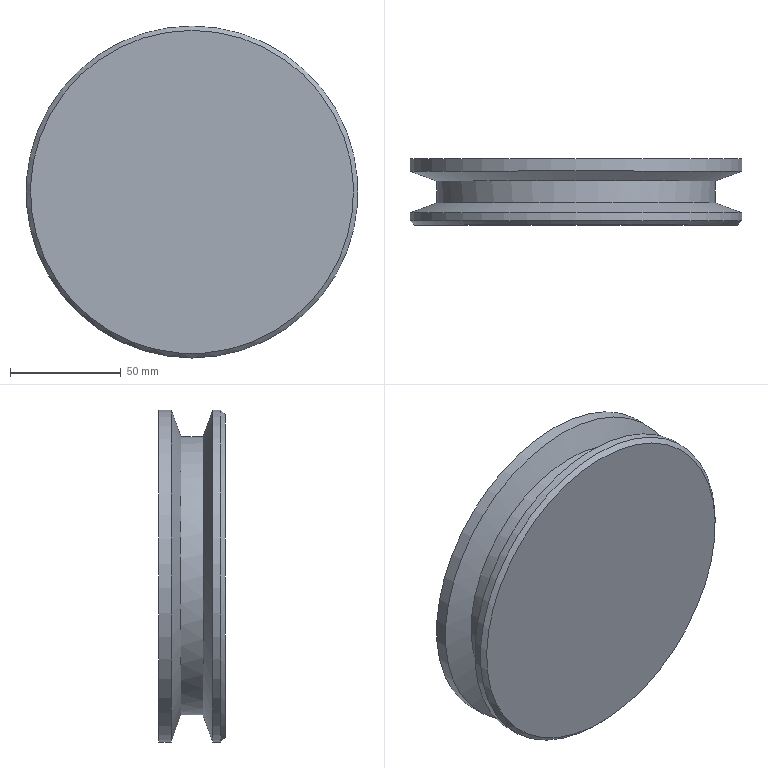Part | STEP file | Tube feed_id134_x_t | 1 solid | 8 faces | box 150 x 30 x 150 mm | volume 453804 mm3 | cylinder 3 | cone 3 | plane 2 | commonest cylinder face diameters 150 x2 126 x1
STEP:
#1=CARTESIAN_POINT('',(0.,0.,0.));
#2=DIRECTION('',(0.,0.,1.));
#3=DIRECTION('',(1.,0.,0.));
#4=AXIS2_PLACEMENT_3D('',#1,#2,#3);
#5=CARTESIAN_POINT('',(-268.5,581.936,-592.5));
#6=VERTEX_POINT('',#5);
#7=CARTESIAN_POINT('',(-268.5,581.936,-665.5));
#8=DIRECTION('',(0.,-1.,0.));
#9=DIRECTION('',(0.,0.,1.));
#10=AXIS2_PLACEMENT_3D('',#7,#8,#9);
#11=CIRCLE('',#10,73.);
#12=CARTESIAN_POINT('',(-268.5,581.936,-665.5));
#13=DIRECTION('',(0.,-1.,0.));
#14=DIRECTION('',(0.,0.,-1.));
#15=AXIS2_PLACEMENT_3D('',#12,#13,#14);
#16=PLANE('',#15);
#17=CARTESIAN_POINT('',(0.,0.));
#18=DIRECTION('',(-1.,0.));
#19=AXIS2_PLACEMENT_2D('',#17,#18);
#20=CIRCLE('',#19,73.);
#21=(GEOMETRIC_REPRESENTATION_CONTEXT(2)PARAMETRIC_REPRESENTATION_CONTEXT()REPRESENTATION_CONTEXT('',''));
#22=DEFINITIONAL_REPRESENTATION('',(#20),#21);
#23=PCURVE('',#16,#22);
#24=CARTESIAN_POINT('',(-268.5,581.936,-665.5));
#25=DIRECTION('',(0.,1.,0.));
#26=DIRECTION('',(0.,0.,-1.));
#27=AXIS2_PLACEMENT_3D('',#24,#25,#26);
#28=CONICAL_SURFACE('',#27,73.,0.7854);
#29=CARTESIAN_POINT('',(9.425,0.));
#30=DIRECTION('',(-1.,0.));
#31=VECTOR('',#30,1.);
#32=LINE('',#29,#31);
#33=(GEOMETRIC_REPRESENTATION_CONTEXT(2)PARAMETRIC_REPRESENTATION_CONTEXT()REPRESENTATION_CONTEXT('',''));
#34=DEFINITIONAL_REPRESENTATION('',(#32),#33);
#35=PCURVE('',#28,#34);
#36=SURFACE_CURVE('',#11,(#23,#35),.PCURVE_S1.);
#37=EDGE_CURVE('',#6,#6,#36,.T.);
#38=ORIENTED_EDGE('',*,*,#37,.T.);
#39=EDGE_LOOP('',(#38));
#40=FACE_BOUND('',#39,.T.);
#41=ADVANCED_FACE('',(#40),#16,.T.);
#42=CARTESIAN_POINT('',(-268.5,611.936,-590.5));
#43=VERTEX_POINT('',#42);
#44=CARTESIAN_POINT('',(-268.5,611.936,-665.5));
#45=DIRECTION('',(0.,-1.,0.));
#46=DIRECTION('',(0.,0.,1.));
#47=AXIS2_PLACEMENT_3D('',#44,#45,#46);
#48=CIRCLE('',#47,75.);
#49=CARTESIAN_POINT('',(-268.5,611.936,-1165.5));
#50=DIRECTION('',(0.,1.,0.));
#51=DIRECTION('',(0.,0.,-1.));
#52=AXIS2_PLACEMENT_3D('',#49,#50,#51);
#53=PLANE('',#52);
#54=CARTESIAN_POINT('',(-575.,0.));
#55=CARTESIAN_POINT('',(-575.,129.904));
#56=CARTESIAN_POINT('',(-462.5,64.952));
#57=CARTESIAN_POINT('',(-350.,0.));
#58=CARTESIAN_POINT('',(-462.5,-64.952));
#59=CARTESIAN_POINT('',(-575.,-129.904));
#60=CARTESIAN_POINT('',(-575.,0.));
#61=(BOUNDED_CURVE()B_SPLINE_CURVE(2,(#54,#55,#56,#57,#58,#59,#60),.UNSPECIFIED.,.T.,.F.)B_SPLINE_CURVE_WITH_KNOTS((1,2,2,2,2,1),(-2.094,0.,2.094,4.189,6.283,8.378),.UNSPECIFIED.)CURVE()GEOMETRIC_REPRESENTATION_ITEM()RATIONAL_B_SPLINE_CURVE((1.,0.5,1.,0.5,1.,0.5,1.))REPRESENTATION_ITEM(''));
#62=(GEOMETRIC_REPRESENTATION_CONTEXT(2)PARAMETRIC_REPRESENTATION_CONTEXT()REPRESENTATION_CONTEXT('',''));
#63=DEFINITIONAL_REPRESENTATION('',(#61),#62);
#64=PCURVE('',#53,#63);
#65=CARTESIAN_POINT('',(-268.5,581.936,-665.5));
#66=DIRECTION('',(0.,1.,0.));
#67=DIRECTION('',(0.,0.,-1.));
#68=AXIS2_PLACEMENT_3D('',#65,#66,#67);
#69=CYLINDRICAL_SURFACE('',#68,75.);
#70=CARTESIAN_POINT('',(9.425,30.));
#71=DIRECTION('',(-1.,0.));
#72=VECTOR('',#71,1.);
#73=LINE('',#70,#72);
#74=(GEOMETRIC_REPRESENTATION_CONTEXT(2)PARAMETRIC_REPRESENTATION_CONTEXT()REPRESENTATION_CONTEXT('',''));
#75=DEFINITIONAL_REPRESENTATION('',(#73),#74);
#76=PCURVE('',#69,#75);
#77=SURFACE_CURVE('',#48,(#64,#76),.PCURVE_S1.);
#78=EDGE_CURVE('',#43,#43,#77,.T.);
#79=ORIENTED_EDGE('',*,*,#78,.F.);
#80=EDGE_LOOP('',(#79));
#81=FACE_BOUND('',#80,.T.);
#82=ADVANCED_FACE('',(#81),#53,.T.);
#83=CARTESIAN_POINT('',(-268.5,606.303,-590.5));
#84=VERTEX_POINT('',#83);
#85=CARTESIAN_POINT('',(-268.5,606.303,-665.5));
#86=DIRECTION('',(0.,1.,0.));
#87=DIRECTION('',(0.,0.,1.));
#88=AXIS2_PLACEMENT_3D('',#85,#86,#87);
#89=CIRCLE('',#88,75.);
#90=CARTESIAN_POINT('',(3.142,24.368));
#91=DIRECTION('',(1.,0.));
#92=VECTOR('',#91,1.);
#93=LINE('',#90,#92);
#94=(GEOMETRIC_REPRESENTATION_CONTEXT(2)PARAMETRIC_REPRESENTATION_CONTEXT()REPRESENTATION_CONTEXT('',''));
#95=DEFINITIONAL_REPRESENTATION('',(#93),#94);
#96=PCURVE('',#69,#95);
#97=CARTESIAN_POINT('',(-268.5,601.936,-665.5));
#98=DIRECTION('',(0.,1.,0.));
#99=DIRECTION('',(0.,0.,1.));
#100=AXIS2_PLACEMENT_3D('',#97,#98,#99);
#101=CONICAL_SURFACE('',#100,63.,1.222);
#102=CARTESIAN_POINT('',(0.,4.368));
#103=DIRECTION('',(1.,0.));
#104=VECTOR('',#103,1.);
#105=LINE('',#102,#104);
#106=(GEOMETRIC_REPRESENTATION_CONTEXT(2)PARAMETRIC_REPRESENTATION_CONTEXT()REPRESENTATION_CONTEXT('',''));
#107=DEFINITIONAL_REPRESENTATION('',(#105),#106);
#108=PCURVE('',#101,#107);
#109=SURFACE_CURVE('',#89,(#96,#108),.PCURVE_S1.);
#110=EDGE_CURVE('',#84,#84,#109,.T.);
#111=ORIENTED_EDGE('',*,*,#110,.T.);
#112=CARTESIAN_POINT('',(-268.5,606.303,-590.5));
#113=CARTESIAN_POINT('',(-268.5,611.936,-590.5));
#114=B_SPLINE_CURVE_WITH_KNOTS('',1,(#112,#113),.UNSPECIFIED.,.F.,.F.,(2,2),(24.368,30.),.PIECEWISE_BEZIER_KNOTS.);
#115=CARTESIAN_POINT('',(9.425,0.));
#116=DIRECTION('',(0.,1.));
#117=VECTOR('',#116,1.);
#118=LINE('',#115,#117);
#119=(GEOMETRIC_REPRESENTATION_CONTEXT(2)PARAMETRIC_REPRESENTATION_CONTEXT()REPRESENTATION_CONTEXT('',''));
#120=DEFINITIONAL_REPRESENTATION('',(#118),#119);
#121=PCURVE('',#69,#120);
#122=CARTESIAN_POINT('',(3.142,0.));
#123=DIRECTION('',(0.,1.));
#124=VECTOR('',#123,1.);
#125=LINE('',#122,#124);
#126=(GEOMETRIC_REPRESENTATION_CONTEXT(2)PARAMETRIC_REPRESENTATION_CONTEXT()REPRESENTATION_CONTEXT('',''));
#127=DEFINITIONAL_REPRESENTATION('',(#125),#126);
#128=PCURVE('',#69,#127);
#129=SEAM_CURVE('',#114,(#121,#128),.PCURVE_S1.);
#130=EDGE_CURVE('',#84,#43,#129,.T.);
#131=ORIENTED_EDGE('',*,*,#130,.T.);
#132=ORIENTED_EDGE('',*,*,#78,.T.);
#133=ORIENTED_EDGE('',*,*,#130,.F.);
#134=EDGE_LOOP('',(#111,#131,#132,#133));
#135=FACE_BOUND('',#134,.T.);
#136=ADVANCED_FACE('',(#135),#69,.T.);
#137=CARTESIAN_POINT('',(-268.5,601.936,-602.5));
#138=VERTEX_POINT('',#137);
#139=CARTESIAN_POINT('',(-268.5,601.936,-665.5));
#140=DIRECTION('',(0.,1.,0.));
#141=DIRECTION('',(0.,0.,1.));
#142=AXIS2_PLACEMENT_3D('',#139,#140,#141);
#143=CIRCLE('',#142,63.);
#144=CARTESIAN_POINT('',(0.,0.));
#145=DIRECTION('',(1.,0.));
#146=VECTOR('',#145,1.);
#147=LINE('',#144,#146);
#148=(GEOMETRIC_REPRESENTATION_CONTEXT(2)PARAMETRIC_REPRESENTATION_CONTEXT()REPRESENTATION_CONTEXT('',''));
#149=DEFINITIONAL_REPRESENTATION('',(#147),#148);
#150=PCURVE('',#101,#149);
#151=CARTESIAN_POINT('',(-268.5,611.936,-665.5));
#152=DIRECTION('',(0.,1.,0.));
#153=DIRECTION('',(0.,0.,1.));
#154=AXIS2_PLACEMENT_3D('',#151,#152,#153);
#155=CYLINDRICAL_SURFACE('',#154,63.);
#156=CARTESIAN_POINT('',(0.,-10.));
#157=DIRECTION('',(1.,0.));
#158=VECTOR('',#157,1.);
#159=LINE('',#156,#158);
#160=(GEOMETRIC_REPRESENTATION_CONTEXT(2)PARAMETRIC_REPRESENTATION_CONTEXT()REPRESENTATION_CONTEXT('',''));
#161=DEFINITIONAL_REPRESENTATION('',(#159),#160);
#162=PCURVE('',#155,#161);
#163=SURFACE_CURVE('',#143,(#150,#162),.PCURVE_S1.);
#164=EDGE_CURVE('',#138,#138,#163,.T.);
#165=ORIENTED_EDGE('',*,*,#164,.T.);
#166=CARTESIAN_POINT('',(-268.5,601.936,-602.5));
#167=CARTESIAN_POINT('',(-268.5,606.303,-590.5));
#168=B_SPLINE_CURVE_WITH_KNOTS('',1,(#166,#167),.UNSPECIFIED.,.F.,.F.,(2,2),(0.,12.77),.PIECEWISE_BEZIER_KNOTS.);
#169=CARTESIAN_POINT('',(6.283,0.));
#170=DIRECTION('',(0.,1.));
#171=VECTOR('',#170,1.);
#172=LINE('',#169,#171);
#173=(GEOMETRIC_REPRESENTATION_CONTEXT(2)PARAMETRIC_REPRESENTATION_CONTEXT()REPRESENTATION_CONTEXT('',''));
#174=DEFINITIONAL_REPRESENTATION('',(#172),#173);
#175=PCURVE('',#101,#174);
#176=CARTESIAN_POINT('',(0.,0.));
#177=DIRECTION('',(0.,1.));
#178=VECTOR('',#177,1.);
#179=LINE('',#176,#178);
#180=(GEOMETRIC_REPRESENTATION_CONTEXT(2)PARAMETRIC_REPRESENTATION_CONTEXT()REPRESENTATION_CONTEXT('',''));
#181=DEFINITIONAL_REPRESENTATION('',(#179),#180);
#182=PCURVE('',#101,#181);
#183=SEAM_CURVE('',#168,(#175,#182),.PCURVE_S1.);
#184=EDGE_CURVE('',#138,#84,#183,.T.);
#185=ORIENTED_EDGE('',*,*,#184,.T.);
#186=ORIENTED_EDGE('',*,*,#110,.F.);
#187=ORIENTED_EDGE('',*,*,#184,.F.);
#188=EDGE_LOOP('',(#165,#185,#186,#187));
#189=FACE_BOUND('',#188,.T.);
#190=ADVANCED_FACE('',(#189),#101,.T.);
#191=ORIENTED_EDGE('',*,*,#164,.F.);
#192=CARTESIAN_POINT('',(-268.5,591.936,-602.5));
#193=VERTEX_POINT('',#192);
#194=CARTESIAN_POINT('',(-268.5,591.936,-602.5));
#195=CARTESIAN_POINT('',(-268.5,601.936,-602.5));
#196=B_SPLINE_CURVE_WITH_KNOTS('',1,(#194,#195),.UNSPECIFIED.,.F.,.F.,(2,2),(-20.,-10.),.PIECEWISE_BEZIER_KNOTS.);
#197=CARTESIAN_POINT('',(0.,0.));
#198=DIRECTION('',(0.,1.));
#199=VECTOR('',#198,1.);
#200=LINE('',#197,#199);
#201=(GEOMETRIC_REPRESENTATION_CONTEXT(2)PARAMETRIC_REPRESENTATION_CONTEXT()REPRESENTATION_CONTEXT('',''));
#202=DEFINITIONAL_REPRESENTATION('',(#200),#201);
#203=PCURVE('',#155,#202);
#204=CARTESIAN_POINT('',(6.283,0.));
#205=DIRECTION('',(0.,1.));
#206=VECTOR('',#205,1.);
#207=LINE('',#204,#206);
#208=(GEOMETRIC_REPRESENTATION_CONTEXT(2)PARAMETRIC_REPRESENTATION_CONTEXT()REPRESENTATION_CONTEXT('',''));
#209=DEFINITIONAL_REPRESENTATION('',(#207),#208);
#210=PCURVE('',#155,#209);
#211=SEAM_CURVE('',#196,(#203,#210),.PCURVE_S1.);
#212=EDGE_CURVE('',#193,#138,#211,.T.);
#213=ORIENTED_EDGE('',*,*,#212,.F.);
#214=CARTESIAN_POINT('',(-268.5,591.936,-728.5));
#215=VERTEX_POINT('',#214);
#216=CARTESIAN_POINT('',(-268.5,591.936,-665.5));
#217=DIRECTION('',(0.,1.,0.));
#218=DIRECTION('',(0.,0.,1.));
#219=AXIS2_PLACEMENT_3D('',#216,#217,#218);
#220=CIRCLE('',#219,63.);
#221=CARTESIAN_POINT('',(0.,-20.));
#222=DIRECTION('',(1.,0.));
#223=VECTOR('',#222,1.);
#224=LINE('',#221,#223);
#225=(GEOMETRIC_REPRESENTATION_CONTEXT(2)PARAMETRIC_REPRESENTATION_CONTEXT()REPRESENTATION_CONTEXT('',''));
#226=DEFINITIONAL_REPRESENTATION('',(#224),#225);
#227=PCURVE('',#155,#226);
#228=CARTESIAN_POINT('',(-268.5,587.568,-665.5));
#229=DIRECTION('',(0.,-1.,0.));
#230=DIRECTION('',(0.,0.,-1.));
#231=AXIS2_PLACEMENT_3D('',#228,#229,#230);
#232=CONICAL_SURFACE('',#231,75.,1.222);
#233=CARTESIAN_POINT('',(3.142,-4.368));
#234=DIRECTION('',(-1.,0.));
#235=VECTOR('',#234,1.);
#236=LINE('',#233,#235);
#237=(GEOMETRIC_REPRESENTATION_CONTEXT(2)PARAMETRIC_REPRESENTATION_CONTEXT()REPRESENTATION_CONTEXT('',''));
#238=DEFINITIONAL_REPRESENTATION('',(#236),#237);
#239=PCURVE('',#232,#238);
#240=SURFACE_CURVE('',#220,(#227,#239),.PCURVE_S1.);
#241=EDGE_CURVE('',#193,#215,#240,.T.);
#242=ORIENTED_EDGE('',*,*,#241,.T.);
#243=CARTESIAN_POINT('',(-268.5,591.936,-665.5));
#244=DIRECTION('',(0.,1.,0.));
#245=DIRECTION('',(0.,0.,1.));
#246=AXIS2_PLACEMENT_3D('',#243,#244,#245);
#247=CIRCLE('',#246,63.);
#248=CARTESIAN_POINT('',(0.,-20.));
#249=DIRECTION('',(1.,0.));
#250=VECTOR('',#249,1.);
#251=LINE('',#248,#250);
#252=(GEOMETRIC_REPRESENTATION_CONTEXT(2)PARAMETRIC_REPRESENTATION_CONTEXT()REPRESENTATION_CONTEXT('',''));
#253=DEFINITIONAL_REPRESENTATION('',(#251),#252);
#254=PCURVE('',#155,#253);
#255=CARTESIAN_POINT('',(9.425,-4.368));
#256=DIRECTION('',(-1.,0.));
#257=VECTOR('',#256,1.);
#258=LINE('',#255,#257);
#259=(GEOMETRIC_REPRESENTATION_CONTEXT(2)PARAMETRIC_REPRESENTATION_CONTEXT()REPRESENTATION_CONTEXT('',''));
#260=DEFINITIONAL_REPRESENTATION('',(#258),#259);
#261=PCURVE('',#232,#260);
#262=SURFACE_CURVE('',#247,(#254,#261),.PCURVE_S1.);
#263=EDGE_CURVE('',#215,#193,#262,.T.);
#264=ORIENTED_EDGE('',*,*,#263,.T.);
#265=ORIENTED_EDGE('',*,*,#212,.T.);
#266=EDGE_LOOP('',(#191,#213,#242,#264,#265));
#267=FACE_BOUND('',#266,.T.);
#268=ADVANCED_FACE('',(#267),#155,.T.);
#269=ORIENTED_EDGE('',*,*,#263,.F.);
#270=CARTESIAN_POINT('',(-268.5,587.568,-740.5));
#271=VERTEX_POINT('',#270);
#272=CARTESIAN_POINT('',(-268.5,591.936,-728.5));
#273=CARTESIAN_POINT('',(-268.5,587.568,-740.5));
#274=B_SPLINE_CURVE_WITH_KNOTS('',1,(#272,#273),.UNSPECIFIED.,.F.,.F.,(2,2),(-12.77,0.),.PIECEWISE_BEZIER_KNOTS.);
#275=CARTESIAN_POINT('',(6.283,0.));
#276=DIRECTION('',(0.,1.));
#277=VECTOR('',#276,1.);
#278=LINE('',#275,#277);
#279=(GEOMETRIC_REPRESENTATION_CONTEXT(2)PARAMETRIC_REPRESENTATION_CONTEXT()REPRESENTATION_CONTEXT('',''));
#280=DEFINITIONAL_REPRESENTATION('',(#278),#279);
#281=PCURVE('',#232,#280);
#282=CARTESIAN_POINT('',(0.,0.));
#283=DIRECTION('',(0.,1.));
#284=VECTOR('',#283,1.);
#285=LINE('',#282,#284);
#286=(GEOMETRIC_REPRESENTATION_CONTEXT(2)PARAMETRIC_REPRESENTATION_CONTEXT()REPRESENTATION_CONTEXT('',''));
#287=DEFINITIONAL_REPRESENTATION('',(#285),#286);
#288=PCURVE('',#232,#287);
#289=SEAM_CURVE('',#274,(#281,#288),.PCURVE_S1.);
#290=EDGE_CURVE('',#215,#271,#289,.T.);
#291=ORIENTED_EDGE('',*,*,#290,.T.);
#292=CARTESIAN_POINT('',(-268.5,587.568,-665.5));
#293=DIRECTION('',(0.,-1.,0.));
#294=DIRECTION('',(0.,0.,-1.));
#295=AXIS2_PLACEMENT_3D('',#292,#293,#294);
#296=CIRCLE('',#295,75.);
#297=CARTESIAN_POINT('',(0.,0.));
#298=DIRECTION('',(1.,0.));
#299=VECTOR('',#298,1.);
#300=LINE('',#297,#299);
#301=(GEOMETRIC_REPRESENTATION_CONTEXT(2)PARAMETRIC_REPRESENTATION_CONTEXT()REPRESENTATION_CONTEXT('',''));
#302=DEFINITIONAL_REPRESENTATION('',(#300),#301);
#303=PCURVE('',#232,#302);
#304=CARTESIAN_POINT('',(-268.5,581.936,-665.5));
#305=DIRECTION('',(0.,1.,0.));
#306=DIRECTION('',(0.,0.,-1.));
#307=AXIS2_PLACEMENT_3D('',#304,#305,#306);
#308=CYLINDRICAL_SURFACE('',#307,75.);
#309=CARTESIAN_POINT('',(6.283,5.632));
#310=DIRECTION('',(-1.,0.));
#311=VECTOR('',#310,1.);
#312=LINE('',#309,#311);
#313=(GEOMETRIC_REPRESENTATION_CONTEXT(2)PARAMETRIC_REPRESENTATION_CONTEXT()REPRESENTATION_CONTEXT('',''));
#314=DEFINITIONAL_REPRESENTATION('',(#312),#313);
#315=PCURVE('',#308,#314);
#316=SURFACE_CURVE('',#296,(#303,#315),.PCURVE_S1.);
#317=EDGE_CURVE('',#271,#271,#316,.T.);
#318=ORIENTED_EDGE('',*,*,#317,.F.);
#319=ORIENTED_EDGE('',*,*,#290,.F.);
#320=ORIENTED_EDGE('',*,*,#241,.F.);
#321=EDGE_LOOP('',(#269,#291,#318,#319,#320));
#322=FACE_BOUND('',#321,.T.);
#323=ADVANCED_FACE('',(#322),#232,.T.);
#324=ORIENTED_EDGE('',*,*,#317,.T.);
#325=CARTESIAN_POINT('',(-268.5,583.936,-740.5));
#326=VERTEX_POINT('',#325);
#327=CARTESIAN_POINT('',(-268.5,583.936,-740.5));
#328=CARTESIAN_POINT('',(-268.5,587.568,-740.5));
#329=B_SPLINE_CURVE_WITH_KNOTS('',1,(#327,#328),.UNSPECIFIED.,.F.,.F.,(2,2),(2.,5.632),.PIECEWISE_BEZIER_KNOTS.);
#330=CARTESIAN_POINT('',(0.,0.));
#331=DIRECTION('',(0.,1.));
#332=VECTOR('',#331,1.);
#333=LINE('',#330,#332);
#334=(GEOMETRIC_REPRESENTATION_CONTEXT(2)PARAMETRIC_REPRESENTATION_CONTEXT()REPRESENTATION_CONTEXT('',''));
#335=DEFINITIONAL_REPRESENTATION('',(#333),#334);
#336=PCURVE('',#308,#335);
#337=CARTESIAN_POINT('',(6.283,0.));
#338=DIRECTION('',(0.,1.));
#339=VECTOR('',#338,1.);
#340=LINE('',#337,#339);
#341=(GEOMETRIC_REPRESENTATION_CONTEXT(2)PARAMETRIC_REPRESENTATION_CONTEXT()REPRESENTATION_CONTEXT('',''));
#342=DEFINITIONAL_REPRESENTATION('',(#340),#341);
#343=PCURVE('',#308,#342);
#344=SEAM_CURVE('',#329,(#336,#343),.PCURVE_S1.);
#345=EDGE_CURVE('',#326,#271,#344,.T.);
#346=ORIENTED_EDGE('',*,*,#345,.F.);
#347=CARTESIAN_POINT('',(-268.5,583.936,-590.5));
#348=VERTEX_POINT('',#347);
#349=CARTESIAN_POINT('',(-268.5,583.936,-665.5));
#350=DIRECTION('',(0.,1.,0.));
#351=DIRECTION('',(0.,0.,1.));
#352=AXIS2_PLACEMENT_3D('',#349,#350,#351);
#353=CIRCLE('',#352,75.);
#354=CARTESIAN_POINT('',(-3.142,2.));
#355=DIRECTION('',(1.,0.));
#356=VECTOR('',#355,1.);
#357=LINE('',#354,#356);
#358=(GEOMETRIC_REPRESENTATION_CONTEXT(2)PARAMETRIC_REPRESENTATION_CONTEXT()REPRESENTATION_CONTEXT('',''));
#359=DEFINITIONAL_REPRESENTATION('',(#357),#358);
#360=PCURVE('',#308,#359);
#361=CARTESIAN_POINT('',(3.142,2.));
#362=DIRECTION('',(1.,0.));
#363=VECTOR('',#362,1.);
#364=LINE('',#361,#363);
#365=(GEOMETRIC_REPRESENTATION_CONTEXT(2)PARAMETRIC_REPRESENTATION_CONTEXT()REPRESENTATION_CONTEXT('',''));
#366=DEFINITIONAL_REPRESENTATION('',(#364),#365);
#367=PCURVE('',#28,#366);
#368=SURFACE_CURVE('',#353,(#360,#367),.PCURVE_S1.);
#369=EDGE_CURVE('',#326,#348,#368,.T.);
#370=ORIENTED_EDGE('',*,*,#369,.T.);
#371=CARTESIAN_POINT('',(-268.5,583.936,-665.5));
#372=DIRECTION('',(0.,1.,0.));
#373=DIRECTION('',(0.,0.,1.));
#374=AXIS2_PLACEMENT_3D('',#371,#372,#373);
#375=CIRCLE('',#374,75.);
#376=CARTESIAN_POINT('',(3.142,2.));
#377=DIRECTION('',(1.,0.));
#378=VECTOR('',#377,1.);
#379=LINE('',#376,#378);
#380=(GEOMETRIC_REPRESENTATION_CONTEXT(2)PARAMETRIC_REPRESENTATION_CONTEXT()REPRESENTATION_CONTEXT('',''));
#381=DEFINITIONAL_REPRESENTATION('',(#379),#380);
#382=PCURVE('',#308,#381);
#383=CARTESIAN_POINT('',(3.142,2.));
#384=DIRECTION('',(1.,0.));
#385=VECTOR('',#384,1.);
#386=LINE('',#383,#385);
#387=(GEOMETRIC_REPRESENTATION_CONTEXT(2)PARAMETRIC_REPRESENTATION_CONTEXT()REPRESENTATION_CONTEXT('',''));
#388=DEFINITIONAL_REPRESENTATION('',(#386),#387);
#389=PCURVE('',#28,#388);
#390=SURFACE_CURVE('',#375,(#382,#389),.PCURVE_S1.);
#391=EDGE_CURVE('',#348,#326,#390,.T.);
#392=ORIENTED_EDGE('',*,*,#391,.T.);
#393=ORIENTED_EDGE('',*,*,#345,.T.);
#394=EDGE_LOOP('',(#324,#346,#370,#392,#393));
#395=FACE_BOUND('',#394,.T.);
#396=ADVANCED_FACE('',(#395),#308,.T.);
#397=ORIENTED_EDGE('',*,*,#391,.F.);
#398=CARTESIAN_POINT('',(-268.5,581.936,-592.5));
#399=CARTESIAN_POINT('',(-268.5,583.936,-590.5));
#400=B_SPLINE_CURVE_WITH_KNOTS('',1,(#398,#399),.UNSPECIFIED.,.F.,.F.,(2,2),(0.,2.828),.PIECEWISE_BEZIER_KNOTS.);
#401=CARTESIAN_POINT('',(3.142,0.));
#402=DIRECTION('',(0.,1.));
#403=VECTOR('',#402,1.);
#404=LINE('',#401,#403);
#405=(GEOMETRIC_REPRESENTATION_CONTEXT(2)PARAMETRIC_REPRESENTATION_CONTEXT()REPRESENTATION_CONTEXT('',''));
#406=DEFINITIONAL_REPRESENTATION('',(#404),#405);
#407=PCURVE('',#28,#406);
#408=CARTESIAN_POINT('',(9.425,0.));
#409=DIRECTION('',(0.,1.));
#410=VECTOR('',#409,1.);
#411=LINE('',#408,#410);
#412=(GEOMETRIC_REPRESENTATION_CONTEXT(2)PARAMETRIC_REPRESENTATION_CONTEXT()REPRESENTATION_CONTEXT('',''));
#413=DEFINITIONAL_REPRESENTATION('',(#411),#412);
#414=PCURVE('',#28,#413);
#415=SEAM_CURVE('',#400,(#407,#414),.PCURVE_S1.);
#416=EDGE_CURVE('',#6,#348,#415,.T.);
#417=ORIENTED_EDGE('',*,*,#416,.F.);
#418=ORIENTED_EDGE('',*,*,#37,.F.);
#419=ORIENTED_EDGE('',*,*,#416,.T.);
#420=ORIENTED_EDGE('',*,*,#369,.F.);
#421=EDGE_LOOP('',(#397,#417,#418,#419,#420));
#422=FACE_BOUND('',#421,.T.);
#423=ADVANCED_FACE('',(#422),#28,.T.);
#424=CLOSED_SHELL('',(#41,#82,#136,#190,#268,#323,#396,#423));
#425=MANIFOLD_SOLID_BREP('',#424);
#426=(LENGTH_UNIT()NAMED_UNIT(*)SI_UNIT(.MILLI.,.METRE.));
#427=UNCERTAINTY_MEASURE_WITH_UNIT(LENGTH_MEASURE(0.00001),#426,'','');
#428=(NAMED_UNIT(*)PLANE_ANGLE_UNIT()SI_UNIT($,.RADIAN.));
#429=(NAMED_UNIT(*)SI_UNIT($,.STERADIAN.)SOLID_ANGLE_UNIT());
#430=(GEOMETRIC_REPRESENTATION_CONTEXT(3)GLOBAL_UNCERTAINTY_ASSIGNED_CONTEXT((#427))GLOBAL_UNIT_ASSIGNED_CONTEXT((#426,#428,#429))REPRESENTATION_CONTEXT('',''));
#431=ADVANCED_BREP_SHAPE_REPRESENTATION('',(#4,#425),#430);